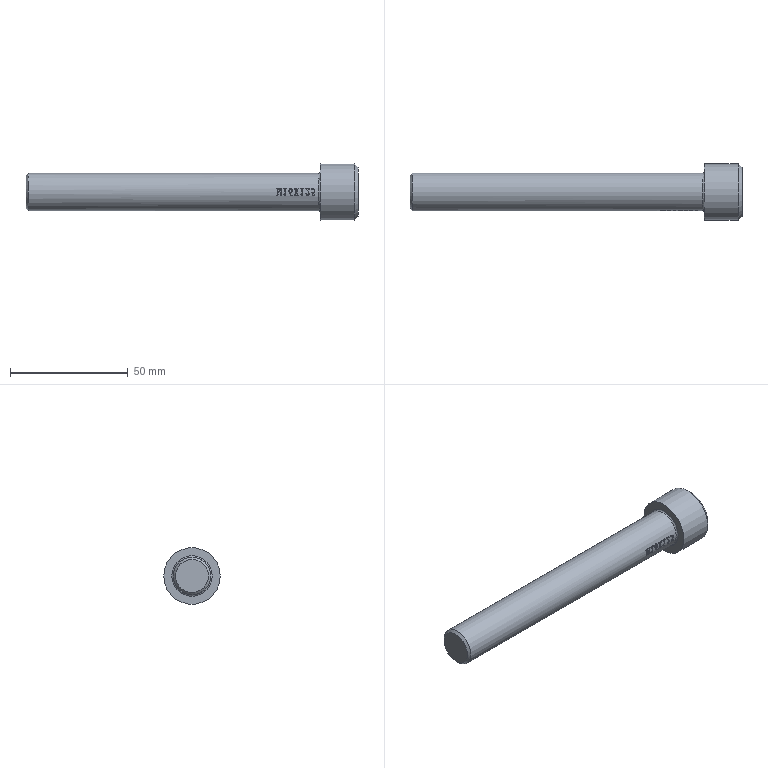Part | STEP file | solid 100 | 1 solid | 121 faces | box 141 x 24 x 24 mm | volume 30892 mm3 | plane 71 | other 38 | sphere 6 | cylinder 3 | cone 2 | torus 1 | commonest cylinder face diameters 16 x2 24 x1